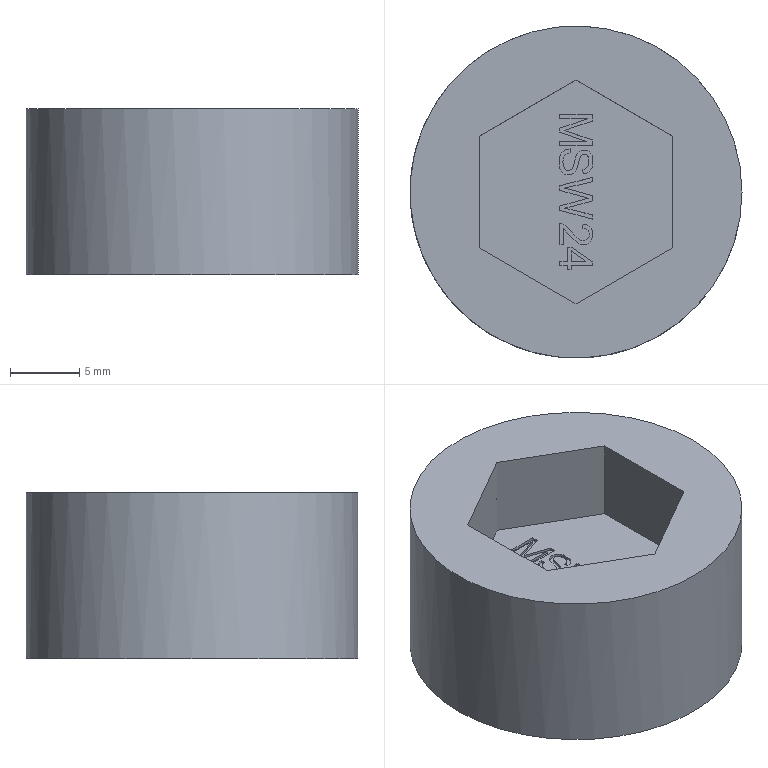Part | NX | features MSW24_1 2 | 1 solid | 103 faces | box 24 x 24 x 12 mm | volume 4408 mm3 | plane 87 | cylinder 16 | commonest cylinder face diameters 0.66 x1 0.684 x1 0.907 x1 0.987 x1 1.1 x1 1.249 x1